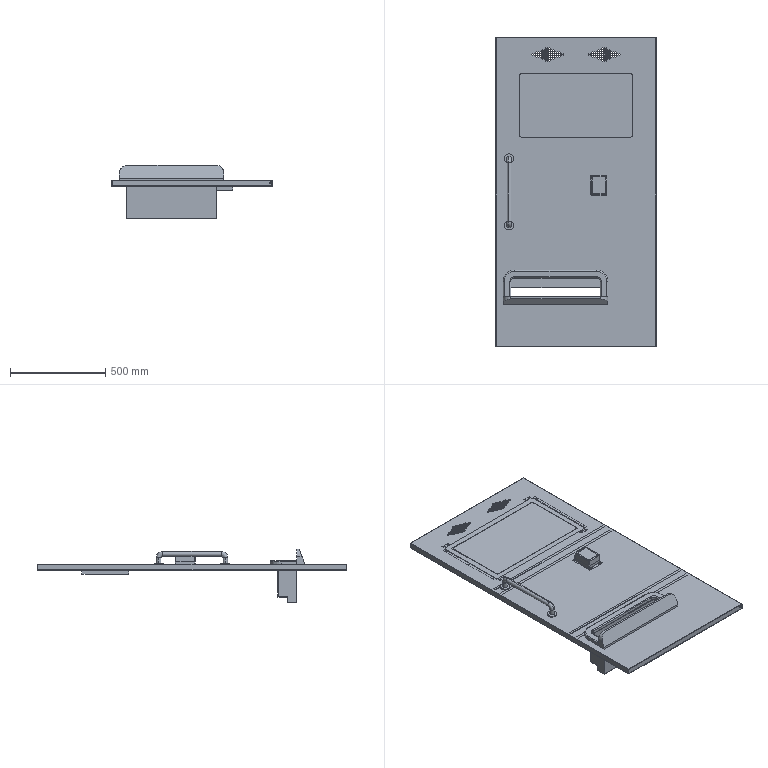Part | SolidWorks | 14 solids | 1385 faces | box 845 x 1628 x 281.2 mm | volume 12737419 mm3 | plane 1109 | cylinder 244 | spline 20 | torus 8 | cone 4 | commonest cylinder face diameters 5 x66 4 x38 2 x34 6 x24 3.2 x20 15 x10